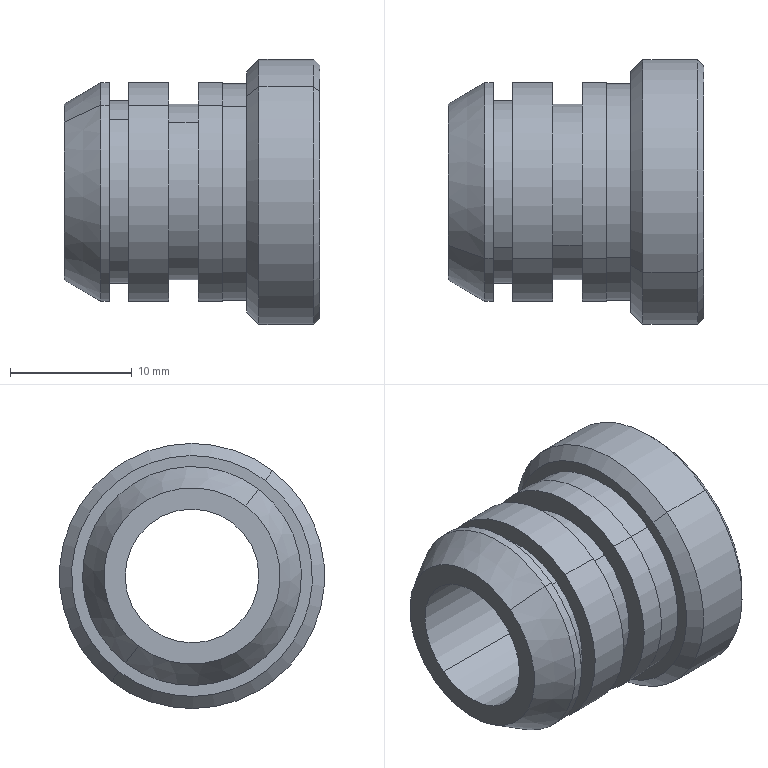Part | SolidWorks | features BaseBody 1 | 1 solid | 35 faces | box 21 x 21.8 x 21.8 mm | volume 3062 mm3 | cylinder 18 | plane 9 | cone 8 | commonest cylinder face diameters 18 x6 11 x2 14.5 x2 15 x2 17 x2 17.8 x2
STEP:
#1=CARTESIAN_POINT('',(-2.263,8.524,-205.203));
#2=VERTEX_POINT('',#1);
#3=CARTESIAN_POINT('',(-2.263,-4.732,-187.897));
#4=VERTEX_POINT('',#3);
#5=CARTESIAN_POINT('',(-2.263,1.896,-196.55));
#6=DIRECTION('',(1.,0.,0.));
#7=DIRECTION('',(0.,0.6081,-0.7939));
#8=AXIS2_PLACEMENT_3D('',#5,#6,#7);
#9=CIRCLE('',#8,10.9);
#10=EDGE_CURVE('',#2,#4,#9,.T.);
#11=ORIENTED_EDGE('',*,*,#10,.T.);
#12=CARTESIAN_POINT('',(2.237,-4.732,-187.897));
#13=VERTEX_POINT('',#12);
#14=CARTESIAN_POINT('',(51.52,-4.732,-187.897));
#15=DIRECTION('',(1.,0.,0.));
#16=VECTOR('',#15,1000.);
#17=LINE('',#14,#16);
#18=EDGE_CURVE('',#4,#13,#17,.T.);
#19=ORIENTED_EDGE('',*,*,#18,.T.);
#20=CARTESIAN_POINT('',(2.237,8.524,-205.203));
#21=VERTEX_POINT('',#20);
#22=CARTESIAN_POINT('',(2.237,1.896,-196.55));
#23=DIRECTION('',(-1.,0.,0.));
#24=DIRECTION('',(0.,-0.6081,0.7939));
#25=AXIS2_PLACEMENT_3D('',#22,#23,#24);
#26=CIRCLE('',#25,10.9);
#27=EDGE_CURVE('',#13,#21,#26,.T.);
#28=ORIENTED_EDGE('',*,*,#27,.T.);
#29=CARTESIAN_POINT('',(51.52,8.524,-205.203));
#30=DIRECTION('',(1.,0.,0.));
#31=VECTOR('',#30,1000.);
#32=LINE('',#29,#31);
#33=EDGE_CURVE('',#2,#21,#32,.T.);
#34=ORIENTED_EDGE('',*,*,#33,.F.);
#35=EDGE_LOOP('',(#11,#19,#28,#34));
#36=FACE_OUTER_BOUND('',#35,.T.);
#37=CARTESIAN_POINT('',(51.52,1.896,-196.55));
#38=DIRECTION('',(1.,0.,0.));
#39=DIRECTION('',(0.,0.6081,-0.7939));
#40=AXIS2_PLACEMENT_3D('',#37,#38,#39);
#41=CYLINDRICAL_SURFACE('',#40,10.9);
#42=ADVANCED_FACE('',(#36),#41,.T.);
#43=CARTESIAN_POINT('',(-5.263,7.308,-203.615));
#44=VERTEX_POINT('',#43);
#45=CARTESIAN_POINT('',(-5.263,-3.516,-189.485));
#46=VERTEX_POINT('',#45);
#47=CARTESIAN_POINT('',(-5.263,1.896,-196.55));
#48=DIRECTION('',(1.,0.,0.));
#49=DIRECTION('',(0.,0.6081,-0.7939));
#50=AXIS2_PLACEMENT_3D('',#47,#48,#49);
#51=CIRCLE('',#50,8.9);
#52=EDGE_CURVE('',#44,#46,#51,.T.);
#53=ORIENTED_EDGE('',*,*,#52,.T.);
#54=CARTESIAN_POINT('',(-3.263,-3.516,-189.485));
#55=VERTEX_POINT('',#54);
#56=CARTESIAN_POINT('',(51.52,-3.516,-189.485));
#57=DIRECTION('',(1.,0.,0.));
#58=VECTOR('',#57,1000.);
#59=LINE('',#56,#58);
#60=EDGE_CURVE('',#46,#55,#59,.T.);
#61=ORIENTED_EDGE('',*,*,#60,.T.);
#62=CARTESIAN_POINT('',(-3.263,7.308,-203.615));
#63=VERTEX_POINT('',#62);
#64=CARTESIAN_POINT('',(-3.263,1.896,-196.55));
#65=DIRECTION('',(1.,0.,0.));
#66=DIRECTION('',(0.,0.6081,-0.7939));
#67=AXIS2_PLACEMENT_3D('',#64,#65,#66);
#68=CIRCLE('',#67,8.9);
#69=EDGE_CURVE('',#63,#55,#68,.T.);
#70=ORIENTED_EDGE('',*,*,#69,.F.);
#71=CARTESIAN_POINT('',(51.52,7.308,-203.615));
#72=DIRECTION('',(1.,0.,0.));
#73=VECTOR('',#72,1000.);
#74=LINE('',#71,#73);
#75=EDGE_CURVE('',#44,#63,#74,.T.);
#76=ORIENTED_EDGE('',*,*,#75,.F.);
#77=EDGE_LOOP('',(#53,#61,#70,#76));
#78=FACE_OUTER_BOUND('',#77,.T.);
#79=CARTESIAN_POINT('',(51.52,1.896,-196.55));
#80=DIRECTION('',(1.,0.,0.));
#81=DIRECTION('',(0.,0.6081,-0.7939));
#82=AXIS2_PLACEMENT_3D('',#79,#80,#81);
#83=CYLINDRICAL_SURFACE('',#82,8.9);
#84=ADVANCED_FACE('',(#78),#83,.T.);
#85=CARTESIAN_POINT('',(-7.263,7.369,-203.695));
#86=VERTEX_POINT('',#85);
#87=CARTESIAN_POINT('',(-7.263,-3.577,-189.405));
#88=VERTEX_POINT('',#87);
#89=CARTESIAN_POINT('',(-7.263,1.896,-196.55));
#90=DIRECTION('',(1.,0.,0.));
#91=DIRECTION('',(0.,0.6081,-0.7939));
#92=AXIS2_PLACEMENT_3D('',#89,#90,#91);
#93=CIRCLE('',#92,9.);
#94=EDGE_CURVE('',#86,#88,#93,.T.);
#95=ORIENTED_EDGE('',*,*,#94,.T.);
#96=CARTESIAN_POINT('',(-5.263,-3.577,-189.405));
#97=VERTEX_POINT('',#96);
#98=CARTESIAN_POINT('',(51.52,-3.577,-189.405));
#99=DIRECTION('',(1.,0.,0.));
#100=VECTOR('',#99,1000.);
#101=LINE('',#98,#100);
#102=EDGE_CURVE('',#88,#97,#101,.T.);
#103=ORIENTED_EDGE('',*,*,#102,.T.);
#104=CARTESIAN_POINT('',(-5.263,7.369,-203.695));
#105=VERTEX_POINT('',#104);
#106=CARTESIAN_POINT('',(-5.263,1.896,-196.55));
#107=DIRECTION('',(1.,0.,0.));
#108=DIRECTION('',(0.,0.6081,-0.7939));
#109=AXIS2_PLACEMENT_3D('',#106,#107,#108);
#110=CIRCLE('',#109,9.);
#111=EDGE_CURVE('',#105,#97,#110,.T.);
#112=ORIENTED_EDGE('',*,*,#111,.F.);
#113=CARTESIAN_POINT('',(51.52,7.369,-203.695));
#114=DIRECTION('',(1.,0.,0.));
#115=VECTOR('',#114,1000.);
#116=LINE('',#113,#115);
#117=EDGE_CURVE('',#86,#105,#116,.T.);
#118=ORIENTED_EDGE('',*,*,#117,.F.);
#119=EDGE_LOOP('',(#95,#103,#112,#118));
#120=FACE_OUTER_BOUND('',#119,.T.);
#121=CARTESIAN_POINT('',(51.52,1.896,-196.55));
#122=DIRECTION('',(1.,0.,0.));
#123=DIRECTION('',(0.,0.6081,-0.7939));
#124=AXIS2_PLACEMENT_3D('',#121,#122,#123);
#125=CYLINDRICAL_SURFACE('',#124,9.);
#126=ADVANCED_FACE('',(#120),#125,.T.);
#127=CARTESIAN_POINT('',(-9.663,6.305,-202.306));
#128=VERTEX_POINT('',#127);
#129=CARTESIAN_POINT('',(-9.663,-2.512,-190.794));
#130=VERTEX_POINT('',#129);
#131=CARTESIAN_POINT('',(-9.663,1.896,-196.55));
#132=DIRECTION('',(1.,0.,0.));
#133=DIRECTION('',(0.,0.6081,-0.7939));
#134=AXIS2_PLACEMENT_3D('',#131,#132,#133);
#135=CIRCLE('',#134,7.25);
#136=EDGE_CURVE('',#128,#130,#135,.T.);
#137=ORIENTED_EDGE('',*,*,#136,.T.);
#138=CARTESIAN_POINT('',(-7.263,-2.512,-190.794));
#139=VERTEX_POINT('',#138);
#140=CARTESIAN_POINT('',(51.52,-2.512,-190.794));
#141=DIRECTION('',(1.,0.,0.));
#142=VECTOR('',#141,1000.);
#143=LINE('',#140,#142);
#144=EDGE_CURVE('',#130,#139,#143,.T.);
#145=ORIENTED_EDGE('',*,*,#144,.T.);
#146=CARTESIAN_POINT('',(-7.263,6.305,-202.306));
#147=VERTEX_POINT('',#146);
#148=CARTESIAN_POINT('',(-7.263,1.896,-196.55));
#149=DIRECTION('',(1.,0.,0.));
#150=DIRECTION('',(0.,0.6081,-0.7939));
#151=AXIS2_PLACEMENT_3D('',#148,#149,#150);
#152=CIRCLE('',#151,7.25);
#153=EDGE_CURVE('',#147,#139,#152,.T.);
#154=ORIENTED_EDGE('',*,*,#153,.F.);
#155=CARTESIAN_POINT('',(51.52,6.305,-202.306));
#156=DIRECTION('',(1.,0.,0.));
#157=VECTOR('',#156,1000.);
#158=LINE('',#155,#157);
#159=EDGE_CURVE('',#128,#147,#158,.T.);
#160=ORIENTED_EDGE('',*,*,#159,.F.);
#161=EDGE_LOOP('',(#137,#145,#154,#160));
#162=FACE_OUTER_BOUND('',#161,.T.);
#163=CARTESIAN_POINT('',(51.52,1.896,-196.55));
#164=DIRECTION('',(1.,0.,0.));
#165=DIRECTION('',(0.,0.6081,-0.7939));
#166=AXIS2_PLACEMENT_3D('',#163,#164,#165);
#167=CYLINDRICAL_SURFACE('',#166,7.25);
#168=ADVANCED_FACE('',(#162),#167,.T.);
#169=CARTESIAN_POINT('',(-12.963,7.369,-203.695));
#170=VERTEX_POINT('',#169);
#171=CARTESIAN_POINT('',(-12.963,-3.577,-189.405));
#172=VERTEX_POINT('',#171);
#173=CARTESIAN_POINT('',(-12.963,1.896,-196.55));
#174=DIRECTION('',(1.,0.,0.));
#175=DIRECTION('',(0.,0.6081,-0.7939));
#176=AXIS2_PLACEMENT_3D('',#173,#174,#175);
#177=CIRCLE('',#176,9.);
#178=EDGE_CURVE('',#170,#172,#177,.T.);
#179=ORIENTED_EDGE('',*,*,#178,.T.);
#180=CARTESIAN_POINT('',(-9.663,-3.577,-189.405));
#181=VERTEX_POINT('',#180);
#182=CARTESIAN_POINT('',(51.52,-3.577,-189.405));
#183=DIRECTION('',(1.,0.,0.));
#184=VECTOR('',#183,1000.);
#185=LINE('',#182,#184);
#186=EDGE_CURVE('',#172,#181,#185,.T.);
#187=ORIENTED_EDGE('',*,*,#186,.T.);
#188=CARTESIAN_POINT('',(-9.663,7.369,-203.695));
#189=VERTEX_POINT('',#188);
#190=CARTESIAN_POINT('',(-9.663,1.896,-196.55));
#191=DIRECTION('',(1.,0.,0.));
#192=DIRECTION('',(0.,0.6081,-0.7939));
#193=AXIS2_PLACEMENT_3D('',#190,#191,#192);
#194=CIRCLE('',#193,9.);
#195=EDGE_CURVE('',#189,#181,#194,.T.);
#196=ORIENTED_EDGE('',*,*,#195,.F.);
#197=CARTESIAN_POINT('',(51.52,7.369,-203.695));
#198=DIRECTION('',(1.,0.,0.));
#199=VECTOR('',#198,1000.);
#200=LINE('',#197,#199);
#201=EDGE_CURVE('',#170,#189,#200,.T.);
#202=ORIENTED_EDGE('',*,*,#201,.F.);
#203=EDGE_LOOP('',(#179,#187,#196,#202));
#204=FACE_OUTER_BOUND('',#203,.T.);
#205=CARTESIAN_POINT('',(51.52,1.896,-196.55));
#206=DIRECTION('',(1.,0.,0.));
#207=DIRECTION('',(0.,0.6081,-0.7939));
#208=AXIS2_PLACEMENT_3D('',#205,#206,#207);
#209=CYLINDRICAL_SURFACE('',#208,9.);
#210=ADVANCED_FACE('',(#204),#209,.T.);
#211=CARTESIAN_POINT('',(-14.563,6.457,-202.504));
#212=VERTEX_POINT('',#211);
#213=CARTESIAN_POINT('',(-14.563,-2.664,-190.596));
#214=VERTEX_POINT('',#213);
#215=CARTESIAN_POINT('',(-14.563,1.896,-196.55));
#216=DIRECTION('',(1.,0.,0.));
#217=DIRECTION('',(0.,0.6081,-0.7939));
#218=AXIS2_PLACEMENT_3D('',#215,#216,#217);
#219=CIRCLE('',#218,7.5);
#220=EDGE_CURVE('',#212,#214,#219,.T.);
#221=ORIENTED_EDGE('',*,*,#220,.T.);
#222=CARTESIAN_POINT('',(-12.963,-2.664,-190.596));
#223=VERTEX_POINT('',#222);
#224=CARTESIAN_POINT('',(51.52,-2.664,-190.596));
#225=DIRECTION('',(1.,0.,0.));
#226=VECTOR('',#225,1000.);
#227=LINE('',#224,#226);
#228=EDGE_CURVE('',#214,#223,#227,.T.);
#229=ORIENTED_EDGE('',*,*,#228,.T.);
#230=CARTESIAN_POINT('',(-12.963,6.457,-202.504));
#231=VERTEX_POINT('',#230);
#232=CARTESIAN_POINT('',(-12.963,1.896,-196.55));
#233=DIRECTION('',(1.,0.,0.));
#234=DIRECTION('',(0.,0.6081,-0.7939));
#235=AXIS2_PLACEMENT_3D('',#232,#233,#234);
#236=CIRCLE('',#235,7.5);
#237=EDGE_CURVE('',#231,#223,#236,.T.);
#238=ORIENTED_EDGE('',*,*,#237,.F.);
#239=CARTESIAN_POINT('',(51.52,6.457,-202.504));
#240=DIRECTION('',(1.,0.,0.));
#241=VECTOR('',#240,1000.);
#242=LINE('',#239,#241);
#243=EDGE_CURVE('',#212,#231,#242,.T.);
#244=ORIENTED_EDGE('',*,*,#243,.F.);
#245=EDGE_LOOP('',(#221,#229,#238,#244));
#246=FACE_OUTER_BOUND('',#245,.T.);
#247=CARTESIAN_POINT('',(51.52,1.896,-196.55));
#248=DIRECTION('',(1.,0.,0.));
#249=DIRECTION('',(0.,0.6081,-0.7939));
#250=AXIS2_PLACEMENT_3D('',#247,#248,#249);
#251=CYLINDRICAL_SURFACE('',#250,7.5);
#252=ADVANCED_FACE('',(#246),#251,.T.);
#253=CARTESIAN_POINT('',(-15.263,7.369,-203.695));
#254=VERTEX_POINT('',#253);
#255=CARTESIAN_POINT('',(-15.263,-3.577,-189.405));
#256=VERTEX_POINT('',#255);
#257=CARTESIAN_POINT('',(-15.263,1.896,-196.55));
#258=DIRECTION('',(1.,0.,0.));
#259=DIRECTION('',(0.,0.6081,-0.7939));
#260=AXIS2_PLACEMENT_3D('',#257,#258,#259);
#261=CIRCLE('',#260,9.);
#262=EDGE_CURVE('',#254,#256,#261,.T.);
#263=ORIENTED_EDGE('',*,*,#262,.T.);
#264=CARTESIAN_POINT('',(-14.563,-3.577,-189.405));
#265=VERTEX_POINT('',#264);
#266=CARTESIAN_POINT('',(51.52,-3.577,-189.405));
#267=DIRECTION('',(1.,0.,0.));
#268=VECTOR('',#267,1000.);
#269=LINE('',#266,#268);
#270=EDGE_CURVE('',#256,#265,#269,.T.);
#271=ORIENTED_EDGE('',*,*,#270,.T.);
#272=CARTESIAN_POINT('',(-14.563,7.369,-203.695));
#273=VERTEX_POINT('',#272);
#274=CARTESIAN_POINT('',(-14.563,1.896,-196.55));
#275=DIRECTION('',(1.,0.,0.));
#276=DIRECTION('',(0.,0.6081,-0.7939));
#277=AXIS2_PLACEMENT_3D('',#274,#275,#276);
#278=CIRCLE('',#277,9.);
#279=EDGE_CURVE('',#273,#265,#278,.T.);
#280=ORIENTED_EDGE('',*,*,#279,.F.);
#281=CARTESIAN_POINT('',(51.52,7.369,-203.695));
#282=DIRECTION('',(1.,0.,0.));
#283=VECTOR('',#282,1000.);
#284=LINE('',#281,#283);
#285=EDGE_CURVE('',#254,#273,#284,.T.);
#286=ORIENTED_EDGE('',*,*,#285,.F.);
#287=EDGE_LOOP('',(#263,#271,#280,#286));
#288=FACE_OUTER_BOUND('',#287,.T.);
#289=CARTESIAN_POINT('',(51.52,1.896,-196.55));
#290=DIRECTION('',(1.,0.,0.));
#291=DIRECTION('',(0.,0.6081,-0.7939));
#292=AXIS2_PLACEMENT_3D('',#289,#290,#291);
#293=CYLINDRICAL_SURFACE('',#292,9.);
#294=ADVANCED_FACE('',(#288),#293,.T.);
#295=CARTESIAN_POINT('',(-18.263,6.305,-202.306));
#296=VERTEX_POINT('',#295);
#297=CARTESIAN_POINT('',(-18.263,-2.512,-190.794));
#298=VERTEX_POINT('',#297);
#299=CARTESIAN_POINT('',(-18.263,1.896,-196.55));
#300=DIRECTION('',(1.,0.,0.));
#301=DIRECTION('',(0.,0.6081,-0.7939));
#302=AXIS2_PLACEMENT_3D('',#299,#300,#301);
#303=CIRCLE('',#302,7.25);
#304=EDGE_CURVE('',#296,#298,#303,.T.);
#305=ORIENTED_EDGE('',*,*,#304,.T.);
#306=CARTESIAN_POINT('',(-18.263,-2.512,-190.794));
#307=DIRECTION('',(0.8638,-0.3064,0.4));
#308=VECTOR('',#307,1000.);
#309=LINE('',#306,#308);
#310=EDGE_CURVE('',#298,#256,#309,.T.);
#311=ORIENTED_EDGE('',*,*,#310,.T.);
#312=ORIENTED_EDGE('',*,*,#262,.F.);
#313=CARTESIAN_POINT('',(-18.263,6.305,-202.306));
#314=DIRECTION('',(0.8638,0.3064,-0.4));
#315=VECTOR('',#314,1000.);
#316=LINE('',#313,#315);
#317=EDGE_CURVE('',#296,#254,#316,.T.);
#318=ORIENTED_EDGE('',*,*,#317,.F.);
#319=EDGE_LOOP('',(#305,#311,#312,#318));
#320=FACE_OUTER_BOUND('',#319,.T.);
#321=CARTESIAN_POINT('',(-18.263,1.896,-196.55));
#322=DIRECTION('',(1.,0.,0.));
#323=DIRECTION('',(0.,0.6081,-0.7939));
#324=AXIS2_PLACEMENT_3D('',#321,#322,#323);
#325=CONICAL_SURFACE('',#324,7.25,0.5281);
#326=ADVANCED_FACE('',(#320),#325,.T.);
#327=CARTESIAN_POINT('',(-18.263,-1.448,-192.184));
#328=VERTEX_POINT('',#327);
#329=CARTESIAN_POINT('',(-18.263,5.241,-200.916));
#330=VERTEX_POINT('',#329);
#331=CARTESIAN_POINT('',(-18.263,1.896,-196.55));
#332=DIRECTION('',(1.,0.,0.));
#333=DIRECTION('',(0.,0.6081,-0.7939));
#334=AXIS2_PLACEMENT_3D('',#331,#332,#333);
#335=CIRCLE('',#334,5.5);
#336=EDGE_CURVE('',#328,#330,#335,.T.);
#337=ORIENTED_EDGE('',*,*,#336,.F.);
#338=CARTESIAN_POINT('',(-0.7629,-1.448,-192.184));
#339=VERTEX_POINT('',#338);
#340=CARTESIAN_POINT('',(51.52,-1.448,-192.184));
#341=DIRECTION('',(1.,0.,0.));
#342=VECTOR('',#341,1000.);
#343=LINE('',#340,#342);
#344=EDGE_CURVE('',#328,#339,#343,.T.);
#345=ORIENTED_EDGE('',*,*,#344,.T.);
#346=CARTESIAN_POINT('',(-0.7629,5.241,-200.916));
#347=VERTEX_POINT('',#346);
#348=CARTESIAN_POINT('',(-0.7629,1.896,-196.55));
#349=DIRECTION('',(1.,0.,0.));
#350=DIRECTION('',(0.,0.6081,-0.7939));
#351=AXIS2_PLACEMENT_3D('',#348,#349,#350);
#352=CIRCLE('',#351,5.5);
#353=EDGE_CURVE('',#339,#347,#352,.T.);
#354=ORIENTED_EDGE('',*,*,#353,.T.);
#355=CARTESIAN_POINT('',(51.52,5.241,-200.916));
#356=DIRECTION('',(1.,0.,0.));
#357=VECTOR('',#356,1000.);
#358=LINE('',#355,#357);
#359=EDGE_CURVE('',#330,#347,#358,.T.);
#360=ORIENTED_EDGE('',*,*,#359,.F.);
#361=EDGE_LOOP('',(#337,#345,#354,#360));
#362=FACE_OUTER_BOUND('',#361,.T.);
#363=CARTESIAN_POINT('',(51.52,1.896,-196.55));
#364=DIRECTION('',(1.,0.,0.));
#365=DIRECTION('',(0.,0.6081,-0.7939));
#366=AXIS2_PLACEMENT_3D('',#363,#364,#365);
#367=CYLINDRICAL_SURFACE('',#366,5.5);
#368=ADVANCED_FACE('',(#362),#367,.F.);
#369=CARTESIAN_POINT('',(-0.7629,-3.273,-189.802));
#370=VERTEX_POINT('',#369);
#371=CARTESIAN_POINT('',(-0.7629,7.065,-203.298));
#372=VERTEX_POINT('',#371);
#373=CARTESIAN_POINT('',(-0.7629,1.896,-196.55));
#374=DIRECTION('',(1.,0.,0.));
#375=DIRECTION('',(0.,0.6081,-0.7939));
#376=AXIS2_PLACEMENT_3D('',#373,#374,#375);
#377=CIRCLE('',#376,8.5);
#378=EDGE_CURVE('',#370,#372,#377,.T.);
#379=ORIENTED_EDGE('',*,*,#378,.F.);
#380=CARTESIAN_POINT('',(2.237,-3.273,-189.802));
#381=VERTEX_POINT('',#380);
#382=CARTESIAN_POINT('',(51.52,-3.273,-189.802));
#383=DIRECTION('',(1.,0.,0.));
#384=VECTOR('',#383,1000.);
#385=LINE('',#382,#384);
#386=EDGE_CURVE('',#370,#381,#385,.T.);
#387=ORIENTED_EDGE('',*,*,#386,.T.);
#388=CARTESIAN_POINT('',(2.237,7.065,-203.298));
#389=VERTEX_POINT('',#388);
#390=CARTESIAN_POINT('',(2.237,1.896,-196.55));
#391=DIRECTION('',(1.,0.,0.));
#392=DIRECTION('',(0.,-0.6081,0.7939));
#393=AXIS2_PLACEMENT_3D('',#390,#391,#392);
#394=CIRCLE('',#393,8.5);
#395=EDGE_CURVE('',#381,#389,#394,.T.);
#396=ORIENTED_EDGE('',*,*,#395,.T.);
#397=CARTESIAN_POINT('',(51.52,7.065,-203.298));
#398=DIRECTION('',(1.,0.,0.));
#399=VECTOR('',#398,1000.);
#400=LINE('',#397,#399);
#401=EDGE_CURVE('',#372,#389,#400,.T.);
#402=ORIENTED_EDGE('',*,*,#401,.F.);
#403=EDGE_LOOP('',(#379,#387,#396,#402));
#404=FACE_OUTER_BOUND('',#403,.T.);
#405=CARTESIAN_POINT('',(51.52,1.896,-196.55));
#406=DIRECTION('',(1.,0.,0.));
#407=DIRECTION('',(0.,0.6081,-0.7939));
#408=AXIS2_PLACEMENT_3D('',#405,#406,#407);
#409=CYLINDRICAL_SURFACE('',#408,8.5);
#410=ADVANCED_FACE('',(#404),#409,.F.);
#411=CARTESIAN_POINT('',(-3.263,-4.124,-188.691));
#412=VERTEX_POINT('',#411);
#413=CARTESIAN_POINT('',(-3.263,7.916,-204.409));
#414=VERTEX_POINT('',#413);
#415=CARTESIAN_POINT('',(-3.263,1.896,-196.55));
#416=DIRECTION('',(-1.,0.,0.));
#417=DIRECTION('',(0.,0.6081,-0.7939));
#418=AXIS2_PLACEMENT_3D('',#415,#416,#417);
#419=CIRCLE('',#418,9.9);
#420=EDGE_CURVE('',#412,#414,#419,.T.);
#421=ORIENTED_EDGE('',*,*,#420,.F.);
#422=CARTESIAN_POINT('',(-2.263,-4.732,-187.897));
#423=DIRECTION('',(0.7071,-0.43,0.5613));
#424=VECTOR('',#423,1000.);
#425=LINE('',#422,#424);
#426=EDGE_CURVE('',#412,#4,#425,.T.);
#427=ORIENTED_EDGE('',*,*,#426,.T.);
#428=ORIENTED_EDGE('',*,*,#10,.F.);
#429=CARTESIAN_POINT('',(-2.263,8.524,-205.203));
#430=DIRECTION('',(0.7071,0.43,-0.5613));
#431=VECTOR('',#430,1000.);
#432=LINE('',#429,#431);
#433=EDGE_CURVE('',#414,#2,#432,.T.);
#434=ORIENTED_EDGE('',*,*,#433,.F.);
#435=EDGE_LOOP('',(#421,#427,#428,#434));
#436=FACE_OUTER_BOUND('',#435,.T.);
#437=CARTESIAN_POINT('',(-2.263,1.896,-196.55));
#438=DIRECTION('',(1.,0.,0.));
#439=DIRECTION('',(0.,0.6081,-0.7939));
#440=AXIS2_PLACEMENT_3D('',#437,#438,#439);
#441=CONICAL_SURFACE('',#440,10.9,0.7854);
#442=ADVANCED_FACE('',(#436),#441,.T.);
#443=ORIENTED_EDGE('',*,*,#395,.F.);
#444=CARTESIAN_POINT('',(2.737,-3.577,-189.405));
#445=VERTEX_POINT('',#444);
#446=CARTESIAN_POINT('',(2.237,-3.273,-189.802));
#447=DIRECTION('',(0.7071,-0.43,0.5613));
#448=VECTOR('',#447,1000.);
#449=LINE('',#446,#448);
#450=EDGE_CURVE('',#381,#445,#449,.T.);
#451=ORIENTED_EDGE('',*,*,#450,.T.);
#452=CARTESIAN_POINT('',(2.737,7.369,-203.695));
#453=VERTEX_POINT('',#452);
#454=CARTESIAN_POINT('',(2.737,1.896,-196.55));
#455=DIRECTION('',(-1.,0.,0.));
#456=DIRECTION('',(0.,-0.6081,0.7939));
#457=AXIS2_PLACEMENT_3D('',#454,#455,#456);
#458=CIRCLE('',#457,9.);
#459=EDGE_CURVE('',#453,#445,#458,.T.);
#460=ORIENTED_EDGE('',*,*,#459,.F.);
#461=CARTESIAN_POINT('',(2.237,7.065,-203.298));
#462=DIRECTION('',(0.7071,0.43,-0.5613));
#463=VECTOR('',#462,1000.);
#464=LINE('',#461,#463);
#465=EDGE_CURVE('',#389,#453,#464,.T.);
#466=ORIENTED_EDGE('',*,*,#465,.F.);
#467=EDGE_LOOP('',(#443,#451,#460,#466));
#468=FACE_OUTER_BOUND('',#467,.T.);
#469=CARTESIAN_POINT('',(2.237,1.896,-196.55));
#470=DIRECTION('',(1.,0.,0.));
#471=DIRECTION('',(0.,0.6081,-0.7939));
#472=AXIS2_PLACEMENT_3D('',#469,#470,#471);
#473=CONICAL_SURFACE('',#472,8.5,0.7854);
#474=ADVANCED_FACE('',(#468),#473,.F.);
#475=CARTESIAN_POINT('',(2.737,8.22,-204.806));
#476=VERTEX_POINT('',#475);
#477=CARTESIAN_POINT('',(2.737,-4.428,-188.294));
#478=VERTEX_POINT('',#477);
#479=CARTESIAN_POINT('',(2.737,1.896,-196.55));
#480=DIRECTION('',(1.,0.,0.));
#481=DIRECTION('',(0.,-0.6081,0.7939));
#482=AXIS2_PLACEMENT_3D('',#479,#480,#481);
#483=CIRCLE('',#482,10.4);
#484=EDGE_CURVE('',#476,#478,#483,.T.);
#485=ORIENTED_EDGE('',*,*,#484,.F.);
#486=CARTESIAN_POINT('',(2.737,8.22,-204.806));
#487=DIRECTION('',(-0.7071,0.43,-0.5613));
#488=VECTOR('',#487,1000.);
#489=LINE('',#486,#488);
#490=EDGE_CURVE('',#476,#21,#489,.T.);
#491=ORIENTED_EDGE('',*,*,#490,.T.);
#492=ORIENTED_EDGE('',*,*,#27,.F.);
#493=CARTESIAN_POINT('',(2.737,-4.428,-188.294));
#494=DIRECTION('',(-0.7071,-0.43,0.5613));
#495=VECTOR('',#494,1000.);
#496=LINE('',#493,#495);
#497=EDGE_CURVE('',#478,#13,#496,.T.);
#498=ORIENTED_EDGE('',*,*,#497,.F.);
#499=EDGE_LOOP('',(#485,#491,#492,#498));
#500=FACE_OUTER_BOUND('',#499,.T.);
#501=CARTESIAN_POINT('',(2.737,1.896,-196.55));
#502=DIRECTION('',(-1.,0.,0.));
#503=DIRECTION('',(0.,-0.6081,0.7939));
#504=AXIS2_PLACEMENT_3D('',#501,#502,#503);
#505=CONICAL_SURFACE('',#504,10.4,0.7854);
#506=ADVANCED_FACE('',(#500),#505,.T.);
#507=ORIENTED_EDGE('',*,*,#490,.F.);
#508=CARTESIAN_POINT('',(2.737,1.896,-196.55));
#509=DIRECTION('',(1.,0.,0.));
#510=DIRECTION('',(0.,-0.6081,0.7939));
#511=AXIS2_PLACEMENT_3D('',#508,#509,#510);
#512=CIRCLE('',#511,10.4);
#513=EDGE_CURVE('',#478,#476,#512,.T.);
#514=ORIENTED_EDGE('',*,*,#513,.F.);
#515=ORIENTED_EDGE('',*,*,#497,.T.);
#516=CARTESIAN_POINT('',(2.237,1.896,-196.55));
#517=DIRECTION('',(-1.,0.,0.));
#518=DIRECTION('',(0.,-0.6081,0.7939));
#519=AXIS2_PLACEMENT_3D('',#516,#517,#518);
#520=CIRCLE('',#519,10.9);
#521=EDGE_CURVE('',#21,#13,#520,.T.);
#522=ORIENTED_EDGE('',*,*,#521,.F.);
#523=EDGE_LOOP('',(#507,#514,#515,#522));
#524=FACE_OUTER_BOUND('',#523,.T.);
#525=CARTESIAN_POINT('',(2.737,1.896,-196.55));
#526=DIRECTION('',(-1.,0.,0.));
#527=DIRECTION('',(0.,-0.6081,0.7939));
#528=AXIS2_PLACEMENT_3D('',#525,#526,#527);
#529=CONICAL_SURFACE('',#528,10.4,0.7854);
#530=ADVANCED_FACE('',(#524),#529,.T.);
#531=ORIENTED_EDGE('',*,*,#450,.F.);
#532=CARTESIAN_POINT('',(2.237,1.896,-196.55));
#533=DIRECTION('',(1.,0.,0.));
#534=DIRECTION('',(0.,-0.6081,0.7939));
#535=AXIS2_PLACEMENT_3D('',#532,#533,#534);
#536=CIRCLE('',#535,8.5);
#537=EDGE_CURVE('',#389,#381,#536,.T.);
#538=ORIENTED_EDGE('',*,*,#537,.F.);
#539=ORIENTED_EDGE('',*,*,#465,.T.);
#540=CARTESIAN_POINT('',(2.737,1.896,-196.55));
#541=DIRECTION('',(-1.,0.,0.));
#542=DIRECTION('',(0.,-0.6081,0.7939));
#543=AXIS2_PLACEMENT_3D('',#540,#541,#542);
#544=CIRCLE('',#543,9.);
#545=EDGE_CURVE('',#445,#453,#544,.T.);
#546=ORIENTED_EDGE('',*,*,#545,.F.);
#547=EDGE_LOOP('',(#531,#538,#539,#546));
#548=FACE_OUTER_BOUND('',#547,.T.);
#549=CARTESIAN_POINT('',(2.237,1.896,-196.55));
#550=DIRECTION('',(1.,0.,0.));
#551=DIRECTION('',(0.,0.6081,-0.7939));
#552=AXIS2_PLACEMENT_3D('',#549,#550,#551);
#553=CONICAL_SURFACE('',#552,8.5,0.7854);
#554=ADVANCED_FACE('',(#548),#553,.F.);
#555=ORIENTED_EDGE('',*,*,#426,.F.);
#556=CARTESIAN_POINT('',(-3.263,1.896,-196.55));
#557=DIRECTION('',(-1.,0.,0.));
#558=DIRECTION('',(0.,0.6081,-0.7939));
#559=AXIS2_PLACEMENT_3D('',#556,#557,#558);
#560=CIRCLE('',#559,9.9);
#561=EDGE_CURVE('',#414,#412,#560,.T.);
#562=ORIENTED_EDGE('',*,*,#561,.F.);
#563=ORIENTED_EDGE('',*,*,#433,.T.);
#564=CARTESIAN_POINT('',(-2.263,1.896,-196.55));
#565=DIRECTION('',(1.,0.,0.));
#566=DIRECTION('',(0.,0.6081,-0.7939));
#567=AXIS2_PLACEMENT_3D('',#564,#565,#566);
#568=CIRCLE('',#567,10.9);
#569=EDGE_CURVE('',#4,#2,#568,.T.);
#570=ORIENTED_EDGE('',*,*,#569,.F.);
#571=EDGE_LOOP('',(#555,#562,#563,#570));
#572=FACE_OUTER_BOUND('',#571,.T.);
#573=CARTESIAN_POINT('',(-2.263,1.896,-196.55));
#574=DIRECTION('',(1.,0.,0.));
#575=DIRECTION('',(0.,0.6081,-0.7939));
#576=AXIS2_PLACEMENT_3D('',#573,#574,#575);
#577=CONICAL_SURFACE('',#576,10.9,0.7854);
#578=ADVANCED_FACE('',(#572),#577,.T.);
#579=ORIENTED_EDGE('',*,*,#513,.T.);
#580=ORIENTED_EDGE('',*,*,#484,.T.);
#581=EDGE_LOOP('',(#579,#580));
#582=FACE_OUTER_BOUND('',#581,.T.);
#583=ORIENTED_EDGE('',*,*,#459,.T.);
#584=ORIENTED_EDGE('',*,*,#545,.T.);
#585=EDGE_LOOP('',(#583,#584));
#586=FACE_BOUND('',#585,.T.);
#587=CARTESIAN_POINT('',(2.737,8.644,-191.381));
#588=DIRECTION('',(-1.,0.,0.));
#589=DIRECTION('',(0.,1.,0.));
#590=AXIS2_PLACEMENT_3D('',#587,#588,#589);
#591=PLANE('',#590);
#592=ADVANCED_FACE('',(#582,#586),#591,.F.);
#593=ORIENTED_EDGE('',*,*,#386,.F.);
#594=CARTESIAN_POINT('',(-0.7629,1.896,-196.55));
#595=DIRECTION('',(1.,0.,0.));
#596=DIRECTION('',(0.,0.6081,-0.7939));
#597=AXIS2_PLACEMENT_3D('',#594,#595,#596);
#598=CIRCLE('',#597,8.5);
#599=EDGE_CURVE('',#372,#370,#598,.T.);
#600=ORIENTED_EDGE('',*,*,#599,.F.);
#601=ORIENTED_EDGE('',*,*,#401,.T.);
#602=ORIENTED_EDGE('',*,*,#537,.T.);
#603=EDGE_LOOP('',(#593,#600,#601,#602));
#604=FACE_OUTER_BOUND('',#603,.T.);
#605=CARTESIAN_POINT('',(51.52,1.896,-196.55));
#606=DIRECTION('',(1.,0.,0.));
#607=DIRECTION('',(0.,0.6081,-0.7939));
#608=AXIS2_PLACEMENT_3D('',#605,#606,#607);
#609=CYLINDRICAL_SURFACE('',#608,8.5);
#610=ADVANCED_FACE('',(#604),#609,.F.);
#611=ORIENTED_EDGE('',*,*,#599,.T.);
#612=ORIENTED_EDGE('',*,*,#378,.T.);
#613=EDGE_LOOP('',(#611,#612));
#614=FACE_OUTER_BOUND('',#613,.T.);
#615=CARTESIAN_POINT('',(-0.7629,1.896,-196.55));
#616=DIRECTION('',(1.,0.,0.));
#617=DIRECTION('',(0.,0.6081,-0.7939));
#618=AXIS2_PLACEMENT_3D('',#615,#616,#617);
#619=CIRCLE('',#618,5.5);
#620=EDGE_CURVE('',#347,#339,#619,.T.);
#621=ORIENTED_EDGE('',*,*,#620,.F.);
#622=ORIENTED_EDGE('',*,*,#353,.F.);
#623=EDGE_LOOP('',(#621,#622));
#624=FACE_BOUND('',#623,.T.);
#625=CARTESIAN_POINT('',(-0.7629,6.262,-193.205));
#626=DIRECTION('',(-1.,0.,0.));
#627=DIRECTION('',(0.,1.,0.));
#628=AXIS2_PLACEMENT_3D('',#625,#626,#627);
#629=PLANE('',#628);
#630=ADVANCED_FACE('',(#614,#624),#629,.F.);
#631=ORIENTED_EDGE('',*,*,#344,.F.);
#632=CARTESIAN_POINT('',(-18.263,1.896,-196.55));
#633=DIRECTION('',(1.,0.,0.));
#634=DIRECTION('',(0.,0.6081,-0.7939));
#635=AXIS2_PLACEMENT_3D('',#632,#633,#634);
#636=CIRCLE('',#635,5.5);
#637=EDGE_CURVE('',#330,#328,#636,.T.);
#638=ORIENTED_EDGE('',*,*,#637,.F.);
#639=ORIENTED_EDGE('',*,*,#359,.T.);
#640=ORIENTED_EDGE('',*,*,#620,.T.);
#641=EDGE_LOOP('',(#631,#638,#639,#640));
#642=FACE_OUTER_BOUND('',#641,.T.);
#643=CARTESIAN_POINT('',(51.52,1.896,-196.55));
#644=DIRECTION('',(1.,0.,0.));
#645=DIRECTION('',(0.,0.6081,-0.7939));
#646=AXIS2_PLACEMENT_3D('',#643,#644,#645);
#647=CYLINDRICAL_SURFACE('',#646,5.5);
#648=ADVANCED_FACE('',(#642),#647,.F.);
#649=ORIENTED_EDGE('',*,*,#637,.T.);
#650=ORIENTED_EDGE('',*,*,#336,.T.);
#651=EDGE_LOOP('',(#649,#650));
#652=FACE_BOUND('',#651,.T.);
#653=ORIENTED_EDGE('',*,*,#304,.F.);
#654=CARTESIAN_POINT('',(-18.263,1.896,-196.55));
#655=DIRECTION('',(1.,0.,0.));
#656=DIRECTION('',(0.,0.6081,-0.7939));
#657=AXIS2_PLACEMENT_3D('',#654,#655,#656);
#658=CIRCLE('',#657,7.25);
#659=EDGE_CURVE('',#298,#296,#658,.T.);
#660=ORIENTED_EDGE('',*,*,#659,.F.);
#661=EDGE_LOOP('',(#653,#660));
#662=FACE_OUTER_BOUND('',#661,.T.);
#663=CARTESIAN_POINT('',(-18.263,7.652,-192.141));
#664=DIRECTION('',(1.,0.,0.));
#665=DIRECTION('',(0.,0.,-1.));
#666=AXIS2_PLACEMENT_3D('',#663,#664,#665);
#667=PLANE('',#666);
#668=ADVANCED_FACE('',(#652,#662),#667,.F.);
#669=ORIENTED_EDGE('',*,*,#310,.F.);
#670=ORIENTED_EDGE('',*,*,#659,.T.);
#671=ORIENTED_EDGE('',*,*,#317,.T.);
#672=CARTESIAN_POINT('',(-15.263,1.896,-196.55));
#673=DIRECTION('',(1.,0.,0.));
#674=DIRECTION('',(0.,0.6081,-0.7939));
#675=AXIS2_PLACEMENT_3D('',#672,#673,#674);
#676=CIRCLE('',#675,9.);
#677=EDGE_CURVE('',#256,#254,#676,.T.);
#678=ORIENTED_EDGE('',*,*,#677,.F.);
#679=EDGE_LOOP('',(#669,#670,#671,#678));
#680=FACE_OUTER_BOUND('',#679,.T.);
#681=CARTESIAN_POINT('',(-18.263,1.896,-196.55));
#682=DIRECTION('',(1.,0.,0.));
#683=DIRECTION('',(0.,0.6081,-0.7939));
#684=AXIS2_PLACEMENT_3D('',#681,#682,#683);
#685=CONICAL_SURFACE('',#684,7.25,0.5281);
#686=ADVANCED_FACE('',(#680),#685,.T.);
#687=ORIENTED_EDGE('',*,*,#270,.F.);
#688=ORIENTED_EDGE('',*,*,#677,.T.);
#689=ORIENTED_EDGE('',*,*,#285,.T.);
#690=CARTESIAN_POINT('',(-14.563,1.896,-196.55));
#691=DIRECTION('',(1.,0.,0.));
#692=DIRECTION('',(0.,0.6081,-0.7939));
#693=AXIS2_PLACEMENT_3D('',#690,#691,#692);
#694=CIRCLE('',#693,9.);
#695=EDGE_CURVE('',#265,#273,#694,.T.);
#696=ORIENTED_EDGE('',*,*,#695,.F.);
#697=EDGE_LOOP('',(#687,#688,#689,#696));
#698=FACE_OUTER_BOUND('',#697,.T.);
#699=CARTESIAN_POINT('',(51.52,1.896,-196.55));
#700=DIRECTION('',(1.,0.,0.));
#701=DIRECTION('',(0.,0.6081,-0.7939));
#702=AXIS2_PLACEMENT_3D('',#699,#700,#701);
#703=CYLINDRICAL_SURFACE('',#702,9.);
#704=ADVANCED_FACE('',(#698),#703,.T.);
#705=ORIENTED_EDGE('',*,*,#279,.T.);
#706=ORIENTED_EDGE('',*,*,#695,.T.);
#707=EDGE_LOOP('',(#705,#706));
#708=FACE_OUTER_BOUND('',#707,.T.);
#709=ORIENTED_EDGE('',*,*,#220,.F.);
#710=CARTESIAN_POINT('',(-14.563,1.896,-196.55));
#711=DIRECTION('',(1.,0.,0.));
#712=DIRECTION('',(0.,0.6081,-0.7939));
#713=AXIS2_PLACEMENT_3D('',#710,#711,#712);
#714=CIRCLE('',#713,7.5);
#715=EDGE_CURVE('',#214,#212,#714,.T.);
#716=ORIENTED_EDGE('',*,*,#715,.F.);
#717=EDGE_LOOP('',(#709,#716));
#718=FACE_BOUND('',#717,.T.);
#719=CARTESIAN_POINT('',(-14.563,7.85,-191.989));
#720=DIRECTION('',(-1.,0.,0.));
#721=DIRECTION('',(0.,1.,0.));
#722=AXIS2_PLACEMENT_3D('',#719,#720,#721);
#723=PLANE('',#722);
#724=ADVANCED_FACE('',(#708,#718),#723,.F.);
#725=ORIENTED_EDGE('',*,*,#228,.F.);
#726=ORIENTED_EDGE('',*,*,#715,.T.);
#727=ORIENTED_EDGE('',*,*,#243,.T.);
#728=CARTESIAN_POINT('',(-12.963,1.896,-196.55));
#729=DIRECTION('',(1.,0.,0.));
#730=DIRECTION('',(0.,0.6081,-0.7939));
#731=AXIS2_PLACEMENT_3D('',#728,#729,#730);
#732=CIRCLE('',#731,7.5);
#733=EDGE_CURVE('',#223,#231,#732,.T.);
#734=ORIENTED_EDGE('',*,*,#733,.F.);
#735=EDGE_LOOP('',(#725,#726,#727,#734));
#736=FACE_OUTER_BOUND('',#735,.T.);
#737=CARTESIAN_POINT('',(51.52,1.896,-196.55));
#738=DIRECTION('',(1.,0.,0.));
#739=DIRECTION('',(0.,0.6081,-0.7939));
#740=AXIS2_PLACEMENT_3D('',#737,#738,#739);
#741=CYLINDRICAL_SURFACE('',#740,7.5);
#742=ADVANCED_FACE('',(#736),#741,.T.);
#743=ORIENTED_EDGE('',*,*,#237,.T.);
#744=ORIENTED_EDGE('',*,*,#733,.T.);
#745=EDGE_LOOP('',(#743,#744));
#746=FACE_BOUND('',#745,.T.);
#747=ORIENTED_EDGE('',*,*,#178,.F.);
#748=CARTESIAN_POINT('',(-12.963,1.896,-196.55));
#749=DIRECTION('',(1.,0.,0.));
#750=DIRECTION('',(0.,0.6081,-0.7939));
#751=AXIS2_PLACEMENT_3D('',#748,#749,#750);
#752=CIRCLE('',#751,9.);
#753=EDGE_CURVE('',#172,#170,#752,.T.);
#754=ORIENTED_EDGE('',*,*,#753,.F.);
#755=EDGE_LOOP('',(#747,#754));
#756=FACE_OUTER_BOUND('',#755,.T.);
#757=CARTESIAN_POINT('',(-12.963,9.041,-191.077));
#758=DIRECTION('',(1.,0.,0.));
#759=DIRECTION('',(0.,0.,-1.));
#760=AXIS2_PLACEMENT_3D('',#757,#758,#759);
#761=PLANE('',#760);
#762=ADVANCED_FACE('',(#746,#756),#761,.F.);
#763=ORIENTED_EDGE('',*,*,#186,.F.);
#764=ORIENTED_EDGE('',*,*,#753,.T.);
#765=ORIENTED_EDGE('',*,*,#201,.T.);
#766=CARTESIAN_POINT('',(-9.663,1.896,-196.55));
#767=DIRECTION('',(1.,0.,0.));
#768=DIRECTION('',(0.,0.6081,-0.7939));
#769=AXIS2_PLACEMENT_3D('',#766,#767,#768);
#770=CIRCLE('',#769,9.);
#771=EDGE_CURVE('',#181,#189,#770,.T.);
#772=ORIENTED_EDGE('',*,*,#771,.F.);
#773=EDGE_LOOP('',(#763,#764,#765,#772));
#774=FACE_OUTER_BOUND('',#773,.T.);
#775=CARTESIAN_POINT('',(51.52,1.896,-196.55));
#776=DIRECTION('',(1.,0.,0.));
#777=DIRECTION('',(0.,0.6081,-0.7939));
#778=AXIS2_PLACEMENT_3D('',#775,#776,#777);
#779=CYLINDRICAL_SURFACE('',#778,9.);
#780=ADVANCED_FACE('',(#774),#779,.T.);
#781=ORIENTED_EDGE('',*,*,#195,.T.);
#782=ORIENTED_EDGE('',*,*,#771,.T.);
#783=EDGE_LOOP('',(#781,#782));
#784=FACE_OUTER_BOUND('',#783,.T.);
#785=ORIENTED_EDGE('',*,*,#136,.F.);
#786=CARTESIAN_POINT('',(-9.663,1.896,-196.55));
#787=DIRECTION('',(1.,0.,0.));
#788=DIRECTION('',(0.,0.6081,-0.7939));
#789=AXIS2_PLACEMENT_3D('',#786,#787,#788);
#790=CIRCLE('',#789,7.25);
#791=EDGE_CURVE('',#130,#128,#790,.T.);
#792=ORIENTED_EDGE('',*,*,#791,.F.);
#793=EDGE_LOOP('',(#785,#792));
#794=FACE_BOUND('',#793,.T.);
#795=CARTESIAN_POINT('',(-9.663,7.652,-192.141));
#796=DIRECTION('',(-1.,0.,0.));
#797=DIRECTION('',(0.,1.,0.));
#798=AXIS2_PLACEMENT_3D('',#795,#796,#797);
#799=PLANE('',#798);
#800=ADVANCED_FACE('',(#784,#794),#799,.F.);
#801=ORIENTED_EDGE('',*,*,#144,.F.);
#802=ORIENTED_EDGE('',*,*,#791,.T.);
#803=ORIENTED_EDGE('',*,*,#159,.T.);
#804=CARTESIAN_POINT('',(-7.263,1.896,-196.55));
#805=DIRECTION('',(1.,0.,0.));
#806=DIRECTION('',(0.,0.6081,-0.7939));
#807=AXIS2_PLACEMENT_3D('',#804,#805,#806);
#808=CIRCLE('',#807,7.25);
#809=EDGE_CURVE('',#139,#147,#808,.T.);
#810=ORIENTED_EDGE('',*,*,#809,.F.);
#811=EDGE_LOOP('',(#801,#802,#803,#810));
#812=FACE_OUTER_BOUND('',#811,.T.);
#813=CARTESIAN_POINT('',(51.52,1.896,-196.55));
#814=DIRECTION('',(1.,0.,0.));
#815=DIRECTION('',(0.,0.6081,-0.7939));
#816=AXIS2_PLACEMENT_3D('',#813,#814,#815);
#817=CYLINDRICAL_SURFACE('',#816,7.25);
#818=ADVANCED_FACE('',(#812),#817,.T.);
#819=ORIENTED_EDGE('',*,*,#153,.T.);
#820=ORIENTED_EDGE('',*,*,#809,.T.);
#821=EDGE_LOOP('',(#819,#820));
#822=FACE_BOUND('',#821,.T.);
#823=ORIENTED_EDGE('',*,*,#94,.F.);
#824=CARTESIAN_POINT('',(-7.263,1.896,-196.55));
#825=DIRECTION('',(1.,0.,0.));
#826=DIRECTION('',(0.,0.6081,-0.7939));
#827=AXIS2_PLACEMENT_3D('',#824,#825,#826);
#828=CIRCLE('',#827,9.);
#829=EDGE_CURVE('',#88,#86,#828,.T.);
#830=ORIENTED_EDGE('',*,*,#829,.F.);
#831=EDGE_LOOP('',(#823,#830));
#832=FACE_OUTER_BOUND('',#831,.T.);
#833=CARTESIAN_POINT('',(-7.263,9.041,-191.077));
#834=DIRECTION('',(1.,0.,0.));
#835=DIRECTION('',(0.,0.,-1.));
#836=AXIS2_PLACEMENT_3D('',#833,#834,#835);
#837=PLANE('',#836);
#838=ADVANCED_FACE('',(#822,#832),#837,.F.);
#839=ORIENTED_EDGE('',*,*,#102,.F.);
#840=ORIENTED_EDGE('',*,*,#829,.T.);
#841=ORIENTED_EDGE('',*,*,#117,.T.);
#842=CARTESIAN_POINT('',(-5.263,1.896,-196.55));
#843=DIRECTION('',(1.,0.,0.));
#844=DIRECTION('',(0.,0.6081,-0.7939));
#845=AXIS2_PLACEMENT_3D('',#842,#843,#844);
#846=CIRCLE('',#845,9.);
#847=EDGE_CURVE('',#97,#105,#846,.T.);
#848=ORIENTED_EDGE('',*,*,#847,.F.);
#849=EDGE_LOOP('',(#839,#840,#841,#848));
#850=FACE_OUTER_BOUND('',#849,.T.);
#851=CARTESIAN_POINT('',(51.52,1.896,-196.55));
#852=DIRECTION('',(1.,0.,0.));
#853=DIRECTION('',(0.,0.6081,-0.7939));
#854=AXIS2_PLACEMENT_3D('',#851,#852,#853);
#855=CYLINDRICAL_SURFACE('',#854,9.);
#856=ADVANCED_FACE('',(#850),#855,.T.);
#857=ORIENTED_EDGE('',*,*,#111,.T.);
#858=ORIENTED_EDGE('',*,*,#847,.T.);
#859=EDGE_LOOP('',(#857,#858));
#860=FACE_OUTER_BOUND('',#859,.T.);
#861=ORIENTED_EDGE('',*,*,#52,.F.);
#862=CARTESIAN_POINT('',(-5.263,1.896,-196.55));
#863=DIRECTION('',(1.,0.,0.));
#864=DIRECTION('',(0.,0.6081,-0.7939));
#865=AXIS2_PLACEMENT_3D('',#862,#863,#864);
#866=CIRCLE('',#865,8.9);
#867=EDGE_CURVE('',#46,#44,#866,.T.);
#868=ORIENTED_EDGE('',*,*,#867,.F.);
#869=EDGE_LOOP('',(#861,#868));
#870=FACE_BOUND('',#869,.T.);
#871=CARTESIAN_POINT('',(-5.263,8.962,-191.138));
#872=DIRECTION('',(-1.,0.,0.));
#873=DIRECTION('',(0.,1.,0.));
#874=AXIS2_PLACEMENT_3D('',#871,#872,#873);
#875=PLANE('',#874);
#876=ADVANCED_FACE('',(#860,#870),#875,.F.);
#877=ORIENTED_EDGE('',*,*,#60,.F.);
#878=ORIENTED_EDGE('',*,*,#867,.T.);
#879=ORIENTED_EDGE('',*,*,#75,.T.);
#880=CARTESIAN_POINT('',(-3.263,1.896,-196.55));
#881=DIRECTION('',(1.,0.,0.));
#882=DIRECTION('',(0.,0.6081,-0.7939));
#883=AXIS2_PLACEMENT_3D('',#880,#881,#882);
#884=CIRCLE('',#883,8.9);
#885=EDGE_CURVE('',#55,#63,#884,.T.);
#886=ORIENTED_EDGE('',*,*,#885,.F.);
#887=EDGE_LOOP('',(#877,#878,#879,#886));
#888=FACE_OUTER_BOUND('',#887,.T.);
#889=CARTESIAN_POINT('',(51.52,1.896,-196.55));
#890=DIRECTION('',(1.,0.,0.));
#891=DIRECTION('',(0.,0.6081,-0.7939));
#892=AXIS2_PLACEMENT_3D('',#889,#890,#891);
#893=CYLINDRICAL_SURFACE('',#892,8.9);
#894=ADVANCED_FACE('',(#888),#893,.T.);
#895=ORIENTED_EDGE('',*,*,#69,.T.);
#896=ORIENTED_EDGE('',*,*,#885,.T.);
#897=EDGE_LOOP('',(#895,#896));
#898=FACE_BOUND('',#897,.T.);
#899=ORIENTED_EDGE('',*,*,#561,.T.);
#900=ORIENTED_EDGE('',*,*,#420,.T.);
#901=EDGE_LOOP('',(#899,#900));
#902=FACE_OUTER_BOUND('',#901,.T.);
#903=CARTESIAN_POINT('',(-3.263,10.549,-189.922));
#904=DIRECTION('',(1.,0.,0.));
#905=DIRECTION('',(0.,0.,-1.));
#906=AXIS2_PLACEMENT_3D('',#903,#904,#905);
#907=PLANE('',#906);
#908=ADVANCED_FACE('',(#898,#902),#907,.F.);
#909=ORIENTED_EDGE('',*,*,#18,.F.);
#910=ORIENTED_EDGE('',*,*,#569,.T.);
#911=ORIENTED_EDGE('',*,*,#33,.T.);
#912=ORIENTED_EDGE('',*,*,#521,.T.);
#913=EDGE_LOOP('',(#909,#910,#911,#912));
#914=FACE_OUTER_BOUND('',#913,.T.);
#915=CARTESIAN_POINT('',(51.52,1.896,-196.55));
#916=DIRECTION('',(1.,0.,0.));
#917=DIRECTION('',(0.,0.6081,-0.7939));
#918=AXIS2_PLACEMENT_3D('',#915,#916,#917);
#919=CYLINDRICAL_SURFACE('',#918,10.9);
#920=ADVANCED_FACE('',(#914),#919,.T.);
#921=CLOSED_SHELL('',(#42,#84,#126,#168,#210,#252,#294,#326,#368,#410,#442,#474,#506,#530,#554,#578,#592,#610,#630,#648,#668,#686,#704,#724,#742,#762,#780,#800,#818,#838,#856,#876,#894,#908,#920));
#922=MANIFOLD_SOLID_BREP('',#921);
#923=CARTESIAN_POINT('',(0.,0.,0.));
#924=DIRECTION('',(0.,0.,1.));
#925=DIRECTION('',(1.,0.,0.));
#926=AXIS2_PLACEMENT_3D('',#923,#924,#925);
#927=(LENGTH_UNIT()NAMED_UNIT(*)SI_UNIT(.MILLI.,.METRE.));
#928=UNCERTAINTY_MEASURE_WITH_UNIT(LENGTH_MEASURE(0.00001),#927,'','');
#929=(NAMED_UNIT(*)PLANE_ANGLE_UNIT()SI_UNIT($,.RADIAN.));
#930=(NAMED_UNIT(*)SI_UNIT($,.STERADIAN.)SOLID_ANGLE_UNIT());
#931=(GEOMETRIC_REPRESENTATION_CONTEXT(3)GLOBAL_UNCERTAINTY_ASSIGNED_CONTEXT((#928))GLOBAL_UNIT_ASSIGNED_CONTEXT((#927,#929,#930))REPRESENTATION_CONTEXT('',''));
#932=ADVANCED_BREP_SHAPE_REPRESENTATION('',(#922,#926),#931);